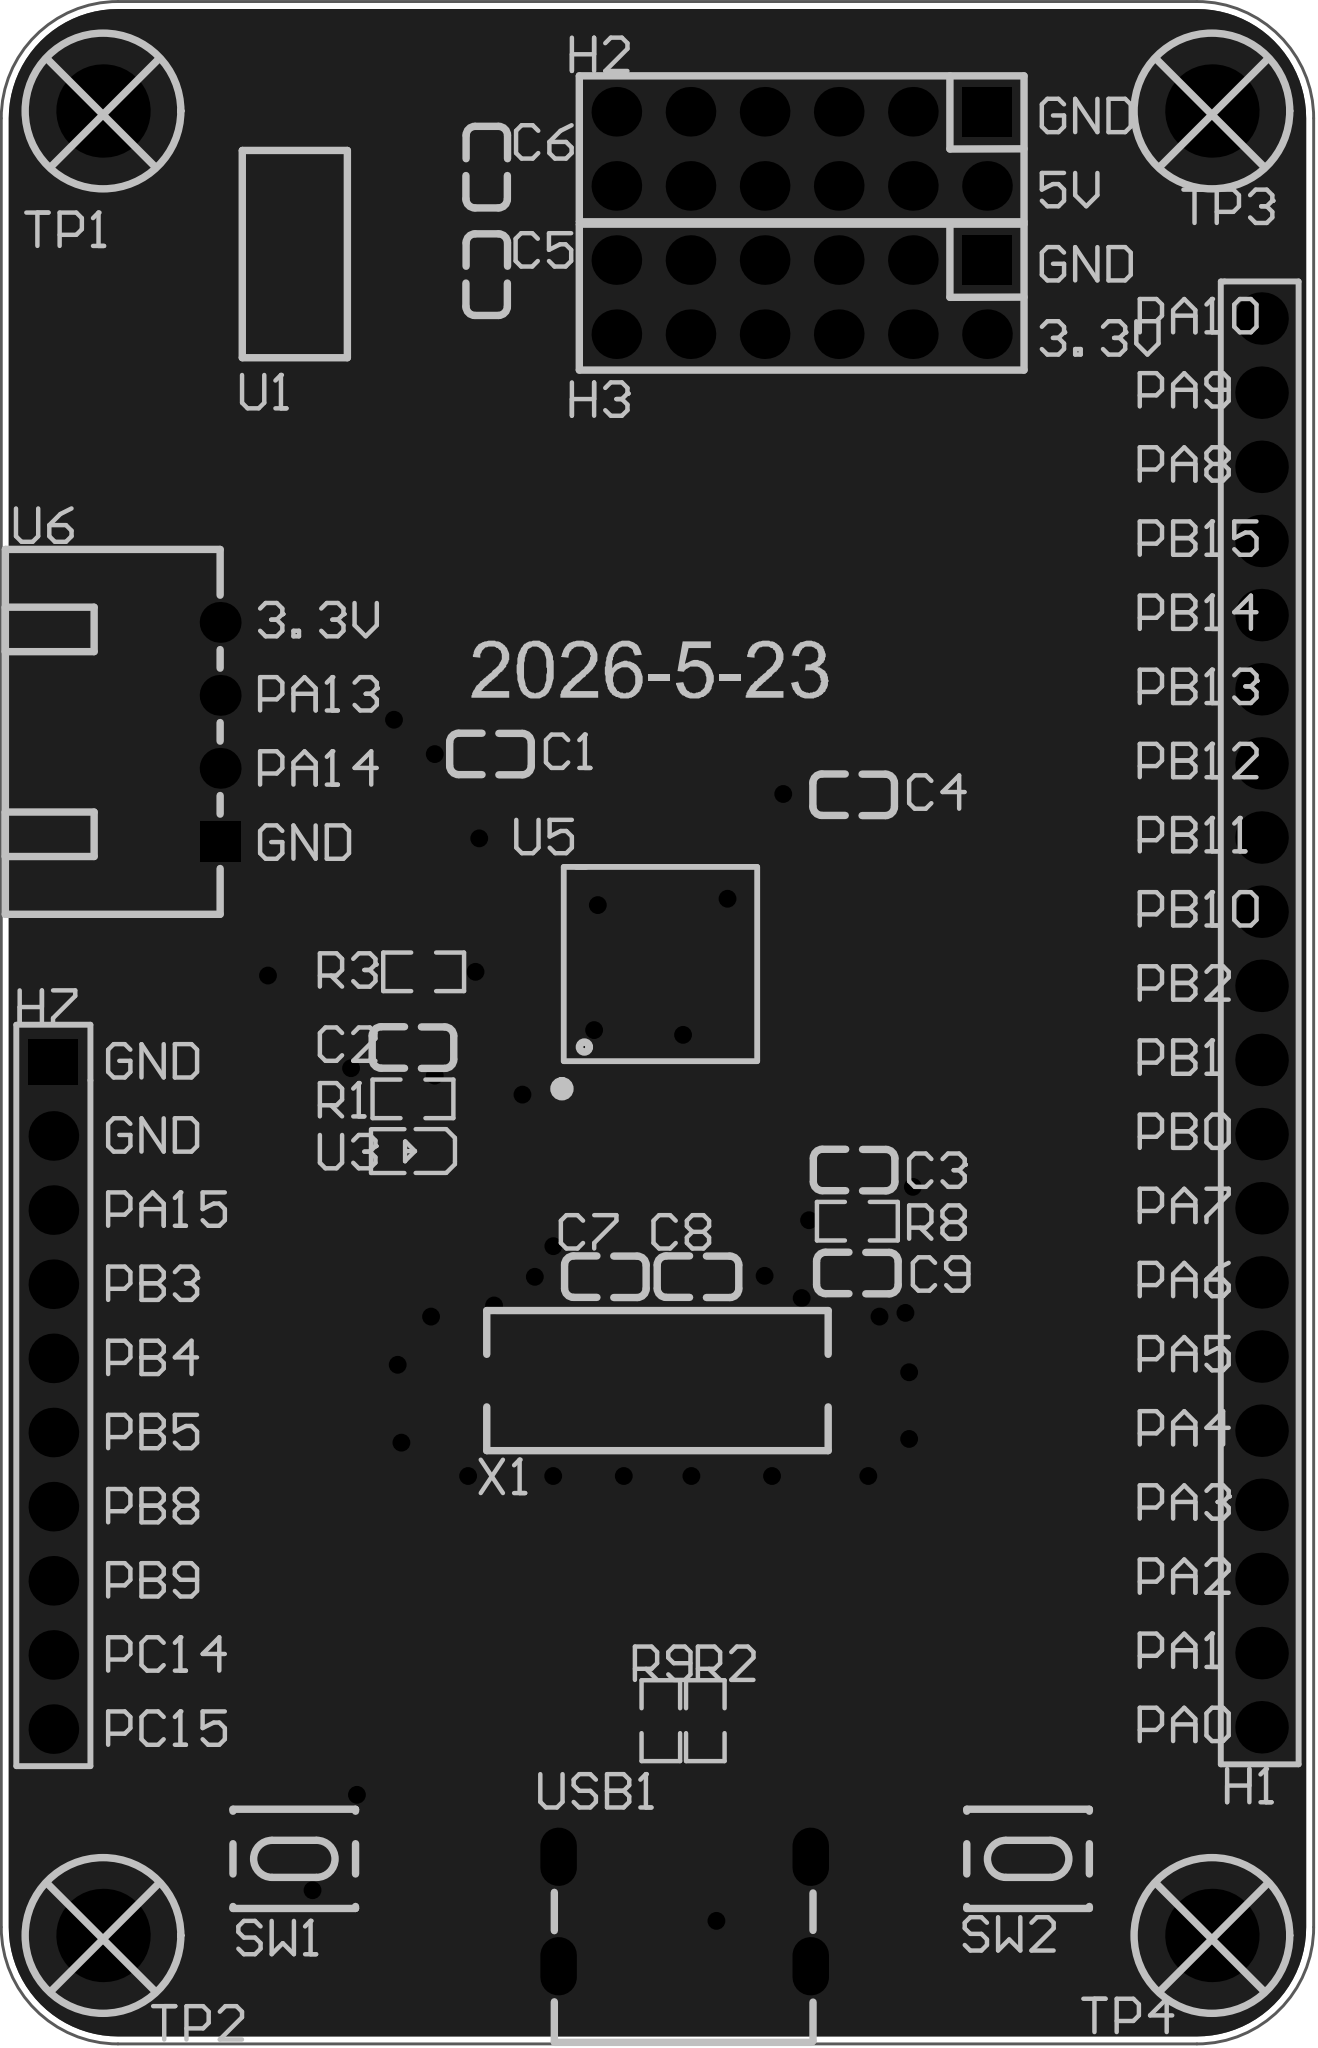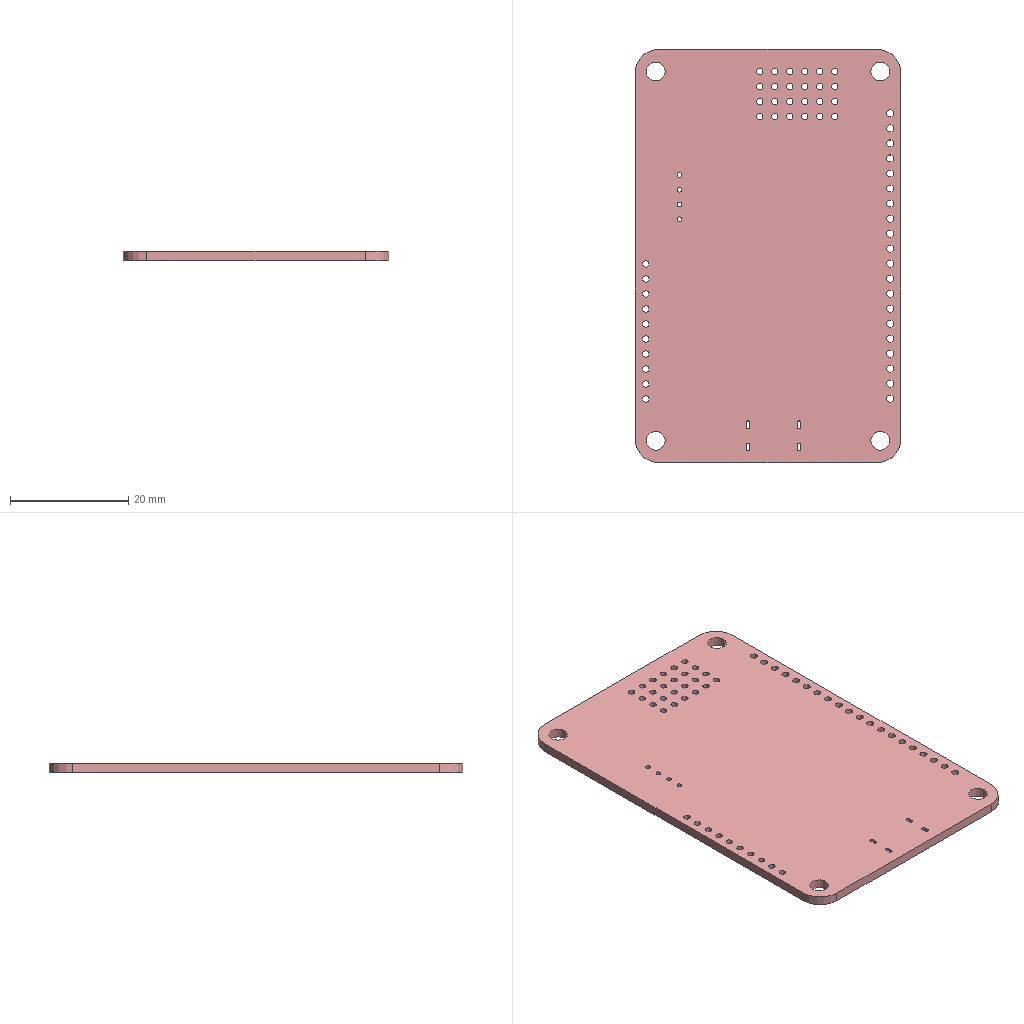Circuit board layout | Altium Designer | box 45 x 70 x 1.6 mm
Layer stack:
# Altium Designer layer stack of  (unit mm; dielectric type: 0 none, 1 core, 2 prepreg, 3 surface material)
index,name,kind,layer,copper_thickness_mm,dielectric_type,dielectric_thickness_mm,dielectric_material,dielectric_constant
0,Top Paste Mask Layer,other,,,,,,
1,Top Silkscreen Layer,other,,,,,,
2,Top Solder Mask Layer,dielectric,,,3,0.01,,3.3
3,Top Layer,copper,Top Layer,0.035,,,,
4,Dielectric1,dielectric,,,3,1.51,FR4,4.5
5,Bottom Layer,copper,Bottom Layer,0.035,,,,
6,Bottom Solder Mask Layer,dielectric,,,3,0.01,,3.3
7,Bottom Silkscreen Layer,other,,,,,,
8,Bottom Paste Mask Layer,other,,,,,,
# drill layer pairs: low layer,high layer
drill_pair,Top Layer,Bottom Layer
Part placement:
Designator,Comment,Layer,Footprint,Center-X(mm),Center-Y(mm),Rotation
SW1,TS-KG89S-AT25F,TopLayer,SW-SMD_4P-L4.2-W3.3-P2.15-LS5.1,92.329,86.995,180
U3,LED_0603,TopLayer,LED_0603,96.347,111.247,180
R3,10K,TopLayer,R0603,96.763,117.382,0
R1,1K,TopLayer,R0603,96.397,113.03,180
C2,100nF,TopLayer,C0603,96.404,114.785,0
C1,100nF,TopLayer,C0603,99.06,124.841,0
X1,8M-HC-49SMD,TopLayer,CRYSTAL-SMD_L11.4-W4.7-LS12.7,104.775,103.378,180
C7,22PF,TopLayer,C0603,102.997,106.934,0
R9,5K1,TopLayer,R0603,104.891,91.728,270
C5,2.2UF,TopLayer,C0603,98.922,141.258,270
C6,10UF,TopLayer,C0603,98.922,144.941,270
C8,22PF,TopLayer,C0603,106.172,106.934,0
C3,100nF,TopLayer,C0603,111.506,110.594,180
C4,100nF,TopLayer,C0603,111.506,123.444,0
R8,10K,TopLayer,R0603,111.625,108.839,0
C9,1UF,TopLayer,C0603,111.633,107.061,0
SW2,TS-KG89S-AT25F,TopLayer,SW-SMD_4P-L4.2-W3.3-P2.15-LS5.1,117.475,86.995,180
H7,,TopLayer,hdr-th_10p-p2.54-v-m-1,84.074,102.87,270
TP1,,TopLayer,M3,85.775,146.872,0
TP2,,TopLayer,M3,85.775,84.37,0
U6,HCZZ0139-4,TopLayer,CONN-TH_4P-P2.50_HCZZ0139-4,89.789,125.603,270
TP4,,TopLayer,M3,123.775,84.37,0
TP3,,TopLayer,M3,123.775,146.872,0
H1,,TopLayer,HDR-TH_20P-P2.54-V-M-1,125.476,115.632,90
R2,5K1,TopLayer,R0603,106.415,91.728,270
U1,,TopLayer,SOT_223,92.348,141.971,90
U5,CH32V203C8T6,TopLayer,LQFP-48_L7.0-W7.0-P0.50-LS9.0-BL,104.891,117.636,0
USB1,,TopLayer,USB__TYPE-C-6P,105.708,85.455,0
H2,,TopLayer,HDR-TH_12P-P2.54-V-M-R2-C6-S2.54,109.717,145.576,180
H3,,TopLayer,HDR-TH_12P-P2.54-V-M-R2-C6-S2.54,109.717,140.496,180
Pad and via stacks:
# Altium Designer via and pad stacks of  (unit mm). Each distinct definition once, with the count of objects using it.
# via: kind,start_layer,end_layer,hole_mm,diameter_mm,mode(0 simple;1 top-mid-bottom;2 full stack),diameter_per_layer,count,example_net
# pad: kind,layer,hole_mm,hole_type(0 round;1 square;2 slot),plating,top_size,top_shape(1 round;2 rect;3 octagon;9 rounded rect),mid_size,bottom_size,mode,footprint,size_per_layer,count,example
pad,Top Layer,0,0,plated,0.7x1.3,2,0.7x1.3,0.7x1.3,0,SW-SMD_4P-L4.2-W3.3-P2.15-LS5.1,,8,SW1.1
pad,Top Layer,0,0,plated,0.8001x0.8001,2,0.8001x0.8001,0.8001x0.8001,0,LED_0603,,2,U3.1
pad,Top Layer,0,0,plated,0.8065x0.864,2,0.8065x0.864,0.8065x0.864,0,R0603,,10,R3.2
pad,Top Layer,0,0,plated,0.8x0.9,2,0.8x0.9,0.8x0.9,0,C0603,,18,C2.2
pad,Top Layer,0,0,plated,5.5x1.4,2,5.5x1.4,5.5x1.4,0,CRYSTAL-SMD_L11.4-W4.7-LS12.7,,2,X1.2
pad,Top Layer,0,0,plated,2.2x3.5,2,2.2x3.5,2.2x3.5,0,SOT_223,,1,U1.4
pad,Top Layer,0,0,plated,1.1x2.2,2,1.1x2.2,1.1x2.2,0,SOT_223,,3,U1.3
pad,Top Layer,0,0,plated,0.27x1.5,1,0.27x1.5,0.27x1.5,0,LQFP-48_L7.0-W7.0-P0.50-LS9.0-BL,,24,U5.1
pad,Top Layer,0,0,plated,1.5x0.27,1,1.5x0.27,1.5x0.27,0,LQFP-48_L7.0-W7.0-P0.50-LS9.0-BL,,24,U5.13
pad,Top Layer,0,0,plated,0.7x1.2,2,0.7x1.2,0.7x1.2,0,USB_ TYPE-C-6P,,2,USB1.A5
pad,Top Layer,0,0,plated,0.8x1.2,2,0.8x1.2,0.8x1.2,0,USB_ TYPE-C-6P,,2,USB1.B9
pad,Top Layer,0,0,plated,0.9x1.2,2,0.9x1.2,0.9x1.2,0,USB_ TYPE-C-6P,,2,USB1.B12
pad,Multi-Layer,1.1,0,plated,1.7x1.7,1,1.7x1.7,1.7x1.7,0,hdr-th_10p-p2.54-v-m-1,,9,H7.10
pad,Multi-Layer,1.1,0,plated,1.575x1.7,2,1.575x1.7,1.575x1.7,0,hdr-th_10p-p2.54-v-m-1,,1,H7.1
pad,Multi-Layer,3.2,0,plated,3.2x3.2,1,3.2x3.2,3.2x3.2,0,M3,,4,TP1.0
pad,Multi-Layer,0.8,0,plated,1.4x1.4,2,1.4x1.4,1.4x1.4,0,CONN-TH_4P-P2.50_HCZZ0139-4,,1,U6.4
pad,Multi-Layer,0.8,0,plated,1.4x1.4,1,1.4x1.4,1.4x1.4,0,CONN-TH_4P-P2.50_HCZZ0139-4,,3,U6.3
pad,Multi-Layer,1.2,0,plated,1.8x1.8,1,1.8x1.8,1.8x1.8,0,HDR-TH_20P-P2.54-V-M-1,,20,H1.20
pad,Multi-Layer,0.6,2,plated,1.25x2,1,1.25x2,1.25x2,0,USB_ TYPE-C-6P,,4,USB1.8
pad,Multi-Layer,1.1,0,plated,1.7x1.7,2,1.7x1.7,1.7x1.7,0,HDR-TH_12P-P2.54-V-M-R2-C6-S2.54,,2,H2.1
pad,Multi-Layer,1.1,0,plated,1.7x1.7,1,1.7x1.7,1.7x1.7,0,HDR-TH_12P-P2.54-V-M-R2-C6-S2.54,,22,H2.2
via,Top Layer,Bottom Layer,0.3048,0.61,0,,36,BOOT0
Copper pours:
name,layer,net,type(0 solid;1 hatched;2 none)
Bottom Layer-GND,Bottom Layer,GND,0
Top Layer-GND,Top Layer,GND,0
Design rules, without the lines most boards share:
# Altium Designer design rules of  (exported by Altium Designer, unit mm)
# columns: name | kind | enabled | priority | scope1 | scope2 | descriptor | typed fields (field=value)
creepage | 65 | enabled | 1 | All | All | Creepage Distance Constraint =(0mil) (All),(All) |